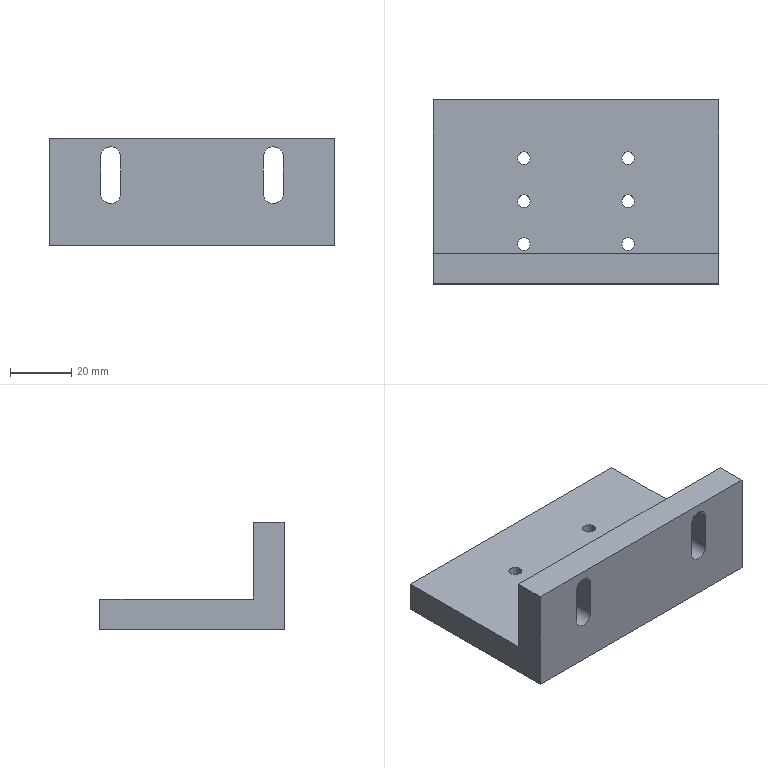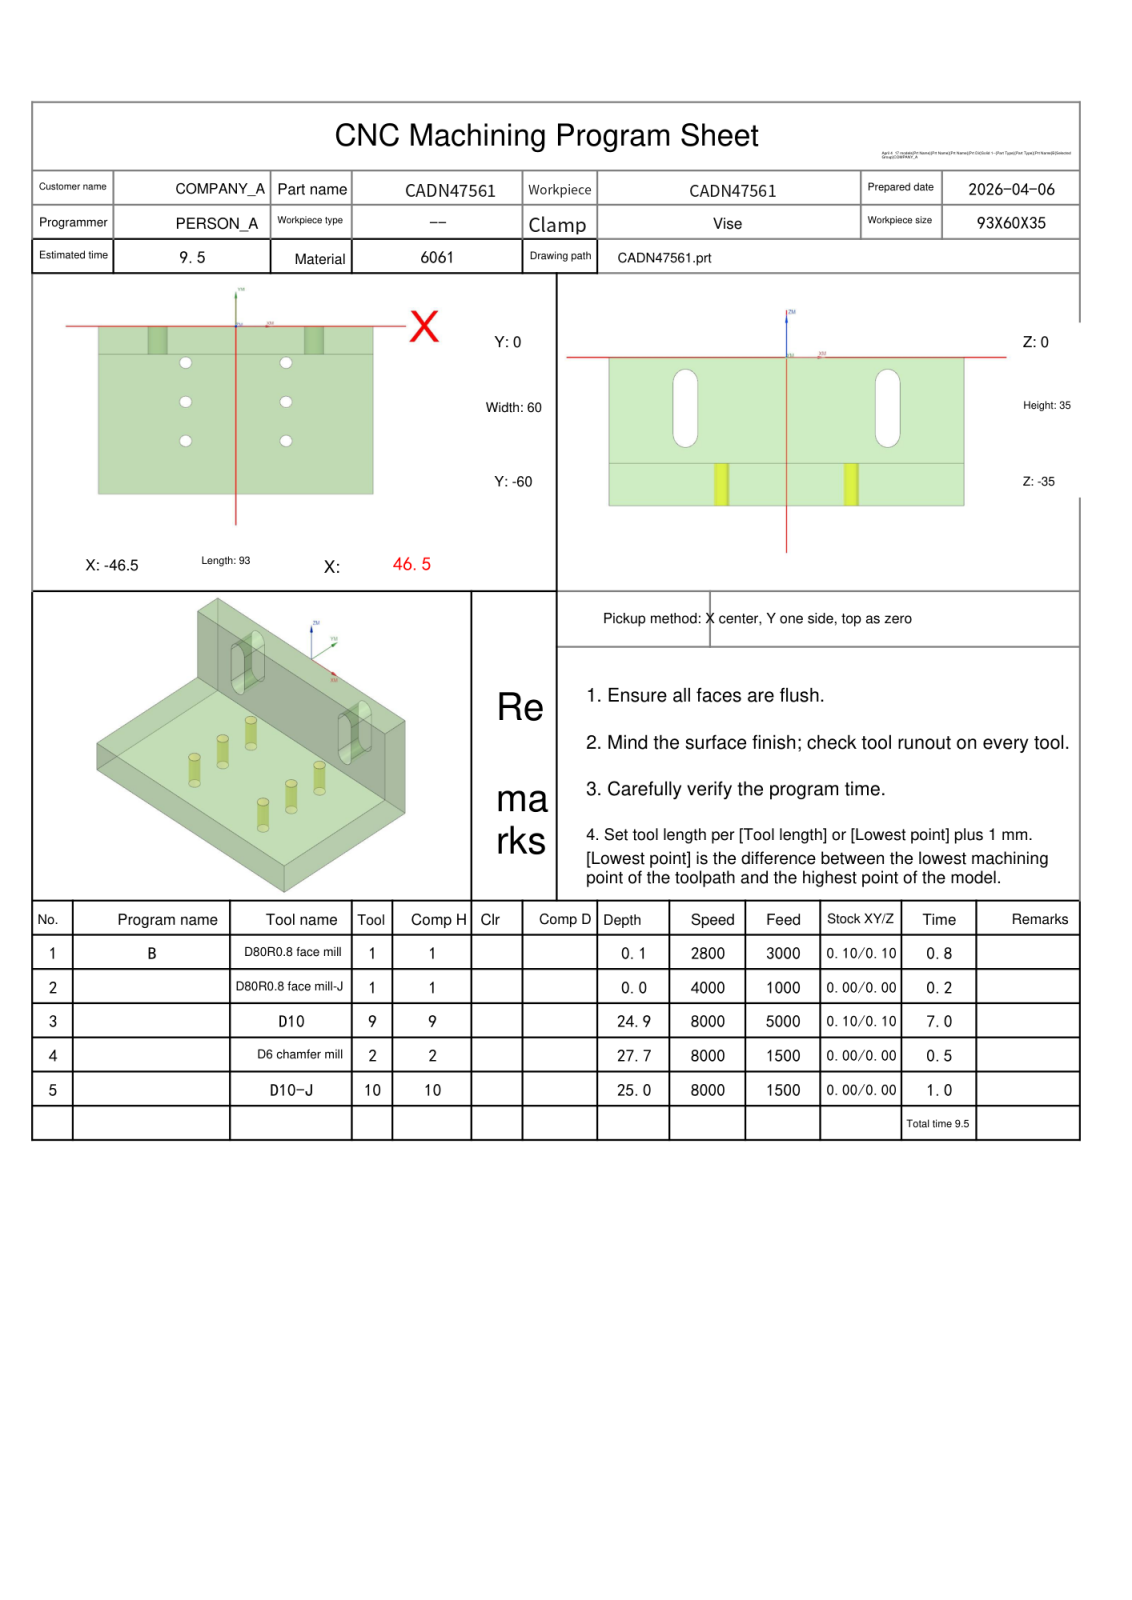NC program | NX | posted by the shop | part box 93 x 60 x 35 mm
Whole program:
%
O0001
(Machine time: 10.28 MIN)
(===Total Tool:4===)
(T1=D80R0.8 face mill D=80.  R=0.8  D-  H01 Z=0.    )
(T9=D10     D=10.  R=0.   D-  H09 Z=-24.9 )
(T2=D6 chamfer mill   D=6.   R=0.   D-  H02 Z=-27.67)
(T10=D10-J  D=10.  R=0.   D10 H10 Z=-25.  )
G80 G90 G17 G49 G40
G91 G28 Z0
M01
N1 T01 M06
(D80R0.8 face mill  D=80. R=0.8 H=01 ce=0.10 di=0.10)
G00 G90 G54 X98.597 Y-30. M03 S2800
G43 H01 Z20.
M08
Z6.011
G01 Z4.011 F3000.
X86.597
X-86.597
X-98.597
Z6.011
G00 X98.597
Z5.522
G01 Z3.522
X86.597
X-86.597
X-98.597
Z5.522
G00 X98.597
Z5.033
G01 Z3.033
X86.597
X-86.597
X-98.597
Z5.033
G00 X98.597
Z4.544
G01 Z2.544
X86.597
X-86.597
X-98.597
Z4.544
G00 Z20.
X98.597
Z4.056
G01 Z2.056
X86.597
X-86.597
X-98.597
Z4.056
G00 Z20.
X98.597
Z3.567
G01 Z1.567
X86.597
X-86.597
X-98.597
Z3.567
G00 Z20.
X98.597
Z3.078
G01 Z1.078
X86.597
X-86.597
X-98.597
Z3.078
G00 Z20.
X98.597
Z2.589
G01 Z.589
X86.597
X-86.597
X-98.597
Z2.589
G00 Z20.
X98.597
Z2.1
G01 Z.1
X86.597
X-86.597
X-98.597
Z2.1
G00 Z20.
G91 G28 Z0.0
M05
M09
G91 G28 Z0.0
M01
N2 T01 M06
(D80R0.8 face mill-J  D=80. R=0.8 H=01 ce=0.00 di=0.00)
G00 G90 G54 X98.499 Y-30. M03 S4000
G43 H01 Z20.
M08
Z2.
G01 Z0.0 F1000.
X86.499
X-86.499
X-98.499
Z2.
G00 Z20.
G91 G28 Z0.0
M05
M09
G91 G28 Z0.0
M01
N3 T09 M06
(D10  D=10. R=0. H=09 ce=0.10 di=0.10)
G00 G90 G54 X54.5 Y-60.1 M03 S8000
G43 H09 Z14.5
M08
Z.907
G01 Z-.593 F5000.
X51.4
X-50.401
G02 X-51.4 Y-59.101 I.001 J1.
G01 Y-53.599
G02 X-50.401 Y-52.6 I1. J-.001
G01 X50.401
G03 X51.4 Y-51.601 I-.001 J1.
G01 Y-46.099
G03 X50.401 Y-45.1 I-1. J-.001
G01 X-50.401
G02 X-51.4 Y-44.101 I.001 J1.
G01 Y-38.599
G02 X-50.401 Y-37.6 I1. J-.001
G01 X50.401
G03 X51.4 Y-36.601 I-.001 J1.
G01 Y-31.099
G03 X50.401 Y-30.1 I-1. J-.001
G01 X-50.401
G02 X-51.4 Y-29.101 I.001 J1.
G01 Y-23.599
G02 X-50.401 Y-22.6 I1. J-.001
G01 X50.544
G03 X51.532 Y-21.755 I-.001 J1.
G01 X52.388 Y-16.254
X52.4 Y-16.1
G03 X51.4 Y-15.1 I-1. J0.0
G01 X-51.4
X-54.6
Z.907
G00 X54.5 Y-60.1
Z.314
G01 Z-1.186
X51.4
X-50.401
G02 X-51.4 Y-59.101 I.001 J1.
G01 Y-53.599
G02 X-50.401 Y-52.6 I1. J-.001
G01 X50.401
G03 X51.4 Y-51.601 I-.001 J1.
G01 Y-46.099
G03 X50.401 Y-45.1 I-1. J-.001
G01 X-50.401
G02 X-51.4 Y-44.101 I.001 J1.
G01 Y-38.599
G02 X-50.401 Y-37.6 I1. J-.001
G01 X50.401
G03 X51.4 Y-36.601 I-.001 J1.
G01 Y-31.099
G03 X50.401 Y-30.1 I-1. J-.001
G01 X-50.401
G02 X-51.4 Y-29.101 I.001 J1.
G01 Y-23.599
G02 X-50.401 Y-22.6 I1. J-.001
G01 X50.544
G03 X51.532 Y-21.755 I-.001 J1.
G01 X52.388 Y-16.254
X52.4 Y-16.1
G03 X51.4 Y-15.1 I-1. J0.0
G01 X-51.4
X-54.6
Z.314
G00 X54.5 Y-60.1
Z-.279
G01 Z-1.779
X51.4
X-50.401
G02 X-51.4 Y-59.101 I.001 J1.
G01 Y-53.599
G02 X-50.401 Y-52.6 I1. J-.001
G01 X50.401
G03 X51.4 Y-51.601 I-.001 J1.
G01 Y-46.099
G03 X50.401 Y-45.1 I-1. J-.001
G01 X-50.401
G02 X-51.4 Y-44.101 I.001 J1.
G01 Y-38.599
G02 X-50.401 Y-37.6 I1. J-.001
G01 X50.401
G03 X51.4 Y-36.601 I-.001 J1.
G01 Y-31.099
G03 X50.401 Y-30.1 I-1. J-.001
G01 X-50.401
G02 X-51.4 Y-29.101 I.001 J1.
G01 Y-23.599
G02 X-50.401 Y-22.6 I1. J-.001
G01 X50.544
G03 X51.532 Y-21.755 I-.001 J1.
G01 X52.388 Y-16.254
X52.4 Y-16.1
G03 X51.4 Y-15.1 I-1. J0.0
G01 X-51.4
X-54.6
Z-.279
G00 X54.5 Y-60.1
Z-.871
G01 Z-2.371
X51.4
X-50.401
G02 X-51.4 Y-59.101 I.001 J1.
G01 Y-53.599
G02 X-50.401 Y-52.6 I1. J-.001
G01 X50.401
G03 X51.4 Y-51.601 I-.001 J1.
G01 Y-46.099
G03 X50.401 Y-45.1 I-1. J-.001
G01 X-50.401
G02 X-51.4 Y-44.101 I.001 J1.
G01 Y-38.599
G02 X-50.401 Y-37.6 I1. J-.001
G01 X50.401
G03 X51.4 Y-36.601 I-.001 J1.
G01 Y-31.099
G03 X50.401 Y-30.1 I-1. J-.001
G01 X-50.401
G02 X-51.4 Y-29.101 I.001 J1.
G01 Y-23.599
G02 X-50.401 Y-22.6 I1. J-.001
G01 X50.544
G03 X51.532 Y-21.755 I-.001 J1.
G01 X52.388 Y-16.254
X52.4 Y-16.1
G03 X51.4 Y-15.1 I-1. J0.0
G01 X-51.4
X-54.6
Z-.871
G00 X54.5 Y-60.1
Z-1.464
G01 Z-2.964
X51.4
X-50.401
G02 X-51.4 Y-59.101 I.001 J1.
G01 Y-53.599
G02 X-50.401 Y-52.6 I1. J-.001
G01 X50.401
G03 X51.4 Y-51.601 I-.001 J1.
G01 Y-46.099
G03 X50.401 Y-45.1 I-1. J-.001
G01 X-50.401
G02 X-51.4 Y-44.101 I.001 J1.
G01 Y-38.599
G02 X-50.401 Y-37.6 I1. J-.001
G01 X50.401
G03 X51.4 Y-36.601 I-.001 J1.
G01 Y-31.099
G03 X50.401 Y-30.1 I-1. J-.001
G01 X-50.401
G02 X-51.4 Y-29.101 I.001 J1.
G01 Y-23.599
G02 X-50.401 Y-22.6 I1. J-.001
G01 X50.544
G03 X51.532 Y-21.755 I-.001 J1.
G01 X52.388 Y-16.254
X52.4 Y-16.1
G03 X51.4 Y-15.1 I-1. J0.0
G01 X-51.4
X-54.6
Z-1.464
G00 X54.5 Y-60.1
Z-2.057
G01 Z-3.557
X51.4
X-50.401
G02 X-51.4 Y-59.101 I.001 J1.
G01 Y-53.599
G02 X-50.401 Y-52.6 I1. J-.001
G01 X50.401
G03 X51.4 Y-51.601 I-.001 J1.
G01 Y-46.099
G03 X50.401 Y-45.1 I-1. J-.001
G01 X-50.401
G02 X-51.4 Y-44.101 I.001 J1.
G01 Y-38.599
G02 X-50.401 Y-37.6 I1. J-.001
G01 X50.401
G03 X51.4 Y-36.601 I-.001 J1.
G01 Y-31.099
G03 X50.401 Y-30.1 I-1. J-.001
G01 X-50.401
G02 X-51.4 Y-29.101 I.001 J1.
G01 Y-23.599
G02 X-50.401 Y-22.6 I1. J-.001
G01 X50.544
G03 X51.532 Y-21.755 I-.001 J1.
G01 X52.388 Y-16.254
X52.4 Y-16.1
G03 X51.4 Y-15.1 I-1. J0.0
G01 X-51.4
X-54.6
Z-2.057
G00 X54.5 Y-60.1
Z-2.65
G01 Z-4.15
X51.4
X-50.401
G02 X-51.4 Y-59.101 I.001 J1.
G01 Y-53.599
G02 X-50.401 Y-52.6 I1. J-.001
G01 X50.401
G03 X51.4 Y-51.601 I-.001 J1.
G01 Y-46.099
G03 X50.401 Y-45.1 I-1. J-.001
G01 X-50.401
G02 X-51.4 Y-44.101 I.001 J1.
G01 Y-38.599
G02 X-50.401 Y-37.6 I1. J-.001
G01 X50.401
G03 X51.4 Y-36.601 I-.001 J1.
G01 Y-31.099
G03 X50.401 Y-30.1 I-1. J-.001
G01 X-50.401
G02 X-51.4 Y-29.101 I.001 J1.
G01 Y-23.599
G02 X-50.401 Y-22.6 I1. J-.001
G01 X50.544
G03 X51.532 Y-21.755 I-.001 J1.
G01 X52.388 Y-16.254
X52.4 Y-16.1
G03 X51.4 Y-15.1 I-1. J0.0
G01 X-51.4
X-54.6
Z-2.65
G00 X54.5 Y-60.1
Z-3.243
G01 Z-4.743
X51.4
X-50.401
G02 X-51.4 Y-59.101 I.001 J1.
G01 Y-53.599
G02 X-50.401 Y-52.6 I1. J-.001
G01 X50.401
G03 X51.4 Y-51.601 I-.001 J1.
G01 Y-46.099
G03 X50.401 Y-45.1 I-1. J-.001
G01 X-50.401
G02 X-51.4 Y-44.101 I.001 J1.
G01 Y-38.599
G02 X-50.401 Y-37.6 I1. J-.001
G01 X50.401
G03 X51.4 Y-36.601 I-.001 J1.
G01 Y-31.099
G03 X50.401 Y-30.1 I-1. J-.001
G01 X-50.401
G02 X-51.4 Y-29.101 I.001 J1.
G01 Y-23.599
G02 X-50.401 Y-22.6 I1. J-.001
G01 X50.544
G03 X51.532 Y-21.755 I-.001 J1.
G01 X52.388 Y-16.254
X52.4 Y-16.1
G03 X51.4 Y-15.1 I-1. J0.0
G01 X-51.4
X-54.6
Z-3.243
G00 X54.5 Y-60.1
Z-3.836
G01 Z-5.336
X51.4
X-50.401
G02 X-51.4 Y-59.101 I.001 J1.
G01 Y-53.599
G02 X-50.401 Y-52.6 I1. J-.001
G01 X50.401
G03 X51.4 Y-51.601 I-.001 J1.
G01 Y-46.099
G03 X50.401 Y-45.1 I-1. J-.001
G01 X-50.401
G02 X-51.4 Y-44.101 I.001 J1.
G01 Y-38.599
G02 X-50.401 Y-37.6 I1. J-.001
G01 X50.401
G03 X51.4 Y-36.601 I-.001 J1.
G01 Y-31.099
G03 X50.401 Y-30.1 I-1. J-.001
G01 X-50.401
G02 X-51.4 Y-29.101 I.001 J1.
G01 Y-23.599
G02 X-50.401 Y-22.6 I1. J-.001
G01 X50.544
G03 X51.532 Y-21.755 I-.001 J1.
G01 X52.388 Y-16.254
X52.4 Y-16.1
G03 X51.4 Y-15.1 I-1. J0.0
G01 X-51.4
X-54.6
Z-3.836
G00 X54.5 Y-60.1
Z-4.429
G01 Z-5.929
X51.4
X-50.401
G02 X-51.4 Y-59.101 I.001 J1.
G01 Y-53.599
G02 X-50.401 Y-52.6 I1. J-.001
G01 X50.401
G03 X51.4 Y-51.601 I-.001 J1.
G01 Y-46.099
G03 X50.401 Y-45.1 I-1. J-.001
G01 X-50.401
G02 X-51.4 Y-44.101 I.001 J1.
G01 Y-38.599
G02 X-50.401 Y-37.6 I1. J-.001
G01 X50.401
G03 X51.4 Y-36.601 I-.001 J1.
G01 Y-31.099
G03 X50.401 Y-30.1 I-1. J-.001
G01 X-50.401
G02 X-51.4 Y-29.101 I.001 J1.
G01 Y-23.599
G02 X-50.401 Y-22.6 I1. J-.001
G01 X50.544
G03 X51.532 Y-21.755 I-.001 J1.
G01 X52.388 Y-16.254
X52.4 Y-16.1
G03 X51.4 Y-15.1 I-1. J0.0
G01 X-51.4
X-54.6
Z-4.429
G00 X54.5 Y-60.1
Z-5.021
G01 Z-6.521
X51.4
X-50.401
G02 X-51.4 Y-59.101 I.001 J1.
G01 Y-53.599
G02 X-50.401 Y-52.6 I1. J-.001
G01 X50.401
G03 X51.4 Y-51.601 I-.001 J1.
G01 Y-46.099
G03 X50.401 Y-45.1 I-1. J-.001
G01 X-50.401
G02 X-51.4 Y-44.101 I.001 J1.
G01 Y-38.599
G02 X-50.401 Y-37.6 I1. J-.001
G01 X50.401
G03 X51.4 Y-36.601 I-.001 J1.
G01 Y-31.099
G03 X50.401 Y-30.1 I-1. J-.001
G01 X-50.401
G02 X-51.4 Y-29.101 I.001 J1.
G01 Y-23.599
G02 X-50.401 Y-22.6 I1. J-.001
G01 X50.544
G03 X51.532 Y-21.755 I-.001 J1.
G01 X52.388 Y-16.254
X52.4 Y-16.1
G03 X51.4 Y-15.1 I-1. J0.0
G01 X-51.4
X-54.6
Z-5.021
G00 X54.5 Y-60.1
Z-5.614
G01 Z-7.114
X51.4
X-50.401
G02 X-51.4 Y-59.101 I.001 J1.
G01 Y-53.599
G02 X-50.401 Y-52.6 I1. J-.001
G01 X50.401
G03 X51.4 Y-51.601 I-.001 J1.
G01 Y-46.099
G03 X50.401 Y-45.1 I-1. J-.001
G01 X-50.401
G02 X-51.4 Y-44.101 I.001 J1.
G01 Y-38.599
G02 X-50.401 Y-37.6 I1. J-.001
G01 X50.401
G03 X51.4 Y-36.601 I-.001 J1.
G01 Y-31.099
G03 X50.401 Y-30.1 I-1. J-.001
G01 X-50.401
G02 X-51.4 Y-29.101 I.001 J1.
G01 Y-23.599
G02 X-50.401 Y-22.6 I1. J-.001
G01 X50.544
G03 X51.532 Y-21.755 I-.001 J1.
G01 X52.388 Y-16.254
X52.4 Y-16.1
G03 X51.4 Y-15.1 I-1. J0.0
G01 X-51.4
X-54.6
Z-5.614
G00 X54.5 Y-60.1
Z-6.207
G01 Z-7.707
X51.4
X-50.401
G02 X-51.4 Y-59.101 I.001 J1.
G01 Y-53.599
G02 X-50.401 Y-52.6 I1. J-.001
G01 X50.401
G03 X51.4 Y-51.601 I-.001 J1.
G01 Y-46.099
G03 X50.401 Y-45.1 I-1. J-.001
G01 X-50.401
G02 X-51.4 Y-44.101 I.001 J1.
G01 Y-38.599
G02 X-50.401 Y-37.6 I1. J-.001
G01 X50.401
G03 X51.4 Y-36.601 I-.001 J1.
G01 Y-31.099
G03 X50.401 Y-30.1 I-1. J-.001
G01 X-50.401
G02 X-51.4 Y-29.101 I.001 J1.
G01 Y-23.599
G02 X-50.401 Y-22.6 I1. J-.001
G01 X50.544
G03 X51.532 Y-21.755 I-.001 J1.
G01 X52.388 Y-16.254
X52.4 Y-16.1
G03 X51.4 Y-15.1 I-1. J0.0
G01 X-51.4
X-54.6
Z-6.207
G00 X54.5 Y-60.1
Z-6.8
G01 Z-8.3
X51.4
X-50.401
G02 X-51.4 Y-59.101 I.001 J1.
G01 Y-53.599
G02 X-50.401 Y-52.6 I1. J-.001
G01 X50.401
G03 X51.4 Y-51.601 I-.001 J1.
G01 Y-46.099
G03 X50.401 Y-45.1 I-1. J-.001
G01 X-50.401
G02 X-51.4 Y-44.101 I.001 J1.
G01 Y-38.599
G02 X-50.401 Y-37.6 I1. J-.001
G01 X50.401
G03 X51.4 Y-36.601 I-.001 J1.
G01 Y-31.099
G03 X50.401 Y-30.1 I-1. J-.001
G01 X-50.401
G02 X-51.4 Y-29.101 I.001 J1.
G01 Y-23.599
G02 X-50.401 Y-22.6 I1. J-.001
G01 X50.544
G03 X51.532 Y-21.755 I-.001 J1.
G01 X52.388 Y-16.254
X52.4 Y-16.1
G03 X51.4 Y-15.1 I-1. J0.0
G01 X-51.4
X-54.6
Z-6.8
G00 X54.5 Y-60.1
Z-7.393
G01 Z-8.893
X51.4
X-50.401
G02 X-51.4 Y-59.101 I.001 J1.
G01 Y-53.599
G02 X-50.401 Y-52.6 I1. J-.001
G01 X50.401
G03 X51.4 Y-51.601 I-.001 J1.
G01 Y-46.099
G03 X50.401 Y-45.1 I-1. J-.001
G01 X-50.401
G02 X-51.4 Y-44.101 I.001 J1.
G01 Y-38.599
G02 X-50.401 Y-37.6 I1. J-.001
G01 X50.401
G03 X51.4 Y-36.601 I-.001 J1.
G01 Y-31.099
G03 X50.401 Y-30.1 I-1. J-.001
G01 X-50.401
G02 X-51.4 Y-29.101 I.001 J1.
G01 Y-23.599
G02 X-50.401 Y-22.6 I1. J-.001
G01 X50.544
G03 X51.532 Y-21.755 I-.001 J1.
G01 X52.388 Y-16.254
X52.4 Y-16.1
G03 X51.4 Y-15.1 I-1. J0.0
G01 X-51.4
X-54.6
Z-7.393
G00 X54.5 Y-60.1
Z-7.986
G01 Z-9.486
X51.4
X-50.401
G02 X-51.4 Y-59.101 I.001 J1.
G01 Y-53.599
G02 X-50.401 Y-52.6 I1. J-.001
G01 X50.401
G03 X51.4 Y-51.601 I-.001 J1.
G01 Y-46.099
G03 X50.401 Y-45.1 I-1. J-.001
G01 X-50.401
G02 X-51.4 Y-44.101 I.001 J1.
G01 Y-38.599
G02 X-50.401 Y-37.6 I1. J-.001
G01 X50.401
G03 X51.4 Y-36.601 I-.001 J1.
G01 Y-31.099
G03 X50.401 Y-30.1 I-1. J-.001
G01 X-50.401
G02 X-51.4 Y-29.101 I.001 J1.
G01 Y-23.599
G02 X-50.401 Y-22.6 I1. J-.001
G01 X50.544
G03 X51.532 Y-21.755 I-.001 J1.
G01 X52.388 Y-16.254
X52.4 Y-16.1
G03 X51.4 Y-15.1 I-1. J0.0
G01 X-51.4
X-54.6
Z-7.986
G00 X54.5 Y-60.1
Z-8.579
G01 Z-10.079
X51.4
X-50.401
G02 X-51.4 Y-59.101 I.001 J1.
G01 Y-53.599
G02 X-50.401 Y-52.6 I1. J-.001
G01 X50.401
G03 X51.4 Y-51.601 I-.001 J1.
G01 Y-46.099
G03 X50.401 Y-45.1 I-1. J-.001
G01 X-50.401
G02 X-51.4 Y-44.101 I.001 J1.
G01 Y-38.599
G02 X-50.401 Y-37.6 I1. J-.001
G01 X50.401
G03 X51.4 Y-36.601 I-.001 J1.
G01 Y-31.099
G03 X50.401 Y-30.1 I-1. J-.001
G01 X-50.401
G02 X-51.4 Y-29.101 I.001 J1.
G01 Y-23.599
G02 X-50.401 Y-22.6 I1. J-.001
G01 X50.544
G03 X51.532 Y-21.755 I-.001 J1.
G01 X52.388 Y-16.254
X52.4 Y-16.1
G03 X51.4 Y-15.1 I-1. J0.0
G01 X-51.4
X-54.6
Z-8.579
G00 X54.5 Y-60.1
Z-9.171
G01 Z-10.671
X51.4
X-50.401
G02 X-51.4 Y-59.101 I.001 J1.
G01 Y-53.599
G02 X-50.401 Y-52.6 I1. J-.001
G01 X50.401
G03 X51.4 Y-51.601 I-.001 J1.
G01 Y-46.099
G03 X50.401 Y-45.1 I-1. J-.001
G01 X-50.401
G02 X-51.4 Y-44.101 I.001 J1.
G01 Y-38.599
G02 X-50.401 Y-37.6 I1. J-.001
G01 X50.401
G03 X51.4 Y-36.601 I-.001 J1.
G01 Y-31.099
G03 X50.401 Y-30.1 I-1. J-.001
G01 X-50.401
G02 X-51.4 Y-29.101 I.001 J1.
G01 Y-23.599
G02 X-50.401 Y-22.6 I1. J-.001
G01 X50.544
G03 X51.532 Y-21.755 I-.001 J1.
G01 X52.388 Y-16.254
X52.4 Y-16.1
G03 X51.4 Y-15.1 I-1. J0.0
G01 X-51.4
X-54.6
Z-9.171
G00 X54.5 Y-60.1
Z-9.764
G01 Z-11.264
X51.4
X-50.401
G02 X-51.4 Y-59.101 I.001 J1.
G01 Y-53.599
G02 X-50.401 Y-52.6 I1. J-.001
G01 X50.401
G03 X51.4 Y-51.601 I-.001 J1.
G01 Y-46.099
G03 X50.401 Y-45.1 I-1. J-.001
G01 X-50.401
G02 X-51.4 Y-44.101 I.001 J1.
G01 Y-38.599
G02 X-50.401 Y-37.6 I1. J-.001
G01 X50.401
G03 X51.4 Y-36.601 I-.001 J1.
G01 Y-31.099
G03 X50.401 Y-30.1 I-1. J-.001
G01 X-50.401
G02 X-51.4 Y-29.101 I.001 J1.
G01 Y-23.599
G02 X-50.401 Y-22.6 I1. J-.001
G01 X50.544
G03 X51.532 Y-21.755 I-.001 J1.
G01 X52.388 Y-16.254
X52.4 Y-16.1
G03 X51.4 Y-15.1 I-1. J0.0
G01 X-51.4
X-54.6
Z-9.764
G00 X54.5 Y-60.1
Z-10.357
G01 Z-11.857
X51.4
X-50.401
G02 X-51.4 Y-59.101 I.001 J1.
G01 Y-53.599
G02 X-50.401 Y-52.6 I1. J-.001
G01 X50.401
G03 X51.4 Y-51.601 I-.001 J1.
G01 Y-46.099
G03 X50.401 Y-45.1 I-1. J-.001
G01 X-50.401
G02 X-51.4 Y-44.101 I.001 J1.
G01 Y-38.599
G02 X-50.401 Y-37.6 I1. J-.001
G01 X50.401
G03 X51.4 Y-36.601 I-.001 J1.
G01 Y-31.099
G03 X50.401 Y-30.1 I-1. J-.001
G01 X-50.401
G02 X-51.4 Y-29.101 I.001 J1.
G01 Y-23.599
G02 X-50.401 Y-22.6 I1. J-.001
G01 X50.544
G03 X51.532 Y-21.755 I-.001 J1.
G01 X52.388 Y-16.254
X52.4 Y-16.1
G03 X51.4 Y-15.1 I-1. J0.0
G01 X-51.4
X-54.6
Z-10.357
G00 X54.5 Y-60.1
Z-10.95
G01 Z-12.45
X51.4
X-50.401
G02 X-51.4 Y-59.101 I.001 J1.
G01 Y-53.599
G02 X-50.401 Y-52.6 I1. J-.001
G01 X50.401
G03 X51.4 Y-51.601 I-.001 J1.
G01 Y-46.099
G03 X50.401 Y-45.1 I-1. J-.001
G01 X-50.401
G02 X-51.4 Y-44.101 I.001 J1.
G01 Y-38.599
G02 X-50.401 Y-37.6 I1. J-.001
G01 X50.401
G03 X51.4 Y-36.601 I-.001 J1.
G01 Y-31.099
G03 X50.401 Y-30.1 I-1. J-.001
G01 X-50.401
G02 X-51.4 Y-29.101 I.001 J1.
G01 Y-23.599
G02 X-50.401 Y-22.6 I1. J-.001
G01 X50.544
G03 X51.532 Y-21.755 I-.001 J1.
G01 X52.388 Y-16.254
X52.4 Y-16.1
G03 X51.4 Y-15.1 I-1. J0.0
G01 X-51.4
X-54.6
Z-10.95
G00 X54.5 Y-60.1
Z-11.543
G01 Z-13.043
X51.4
X-50.401
G02 X-51.4 Y-59.101 I.001 J1.
G01 Y-53.599
G02 X-50.401 Y-52.6 I1. J-.001
G01 X50.401
G03 X51.4 Y-51.601 I-.001 J1.
G01 Y-46.099
G03 X50.401 Y-45.1 I-1. J-.001
G01 X-50.401
G02 X-51.4 Y-44.101 I.001 J1.
G01 Y-38.599
G02 X-50.401 Y-37.6 I1. J-.001
G01 X50.401
G03 X51.4 Y-36.601 I-.001 J1.
G01 Y-31.099
G03 X50.401 Y-30.1 I-1. J-.001
G01 X-50.401
G02 X-51.4 Y-29.101 I.001 J1.
G01 Y-23.599
G02 X-50.401 Y-22.6 I1. J-.001
G01 X50.544
G03 X51.532 Y-21.755 I-.001 J1.
G01 X52.388 Y-16.254
X52.4 Y-16.1
G03 X51.4 Y-15.1 I-1. J0.0
G01 X-51.4
X-54.6
Z-11.543
G00 X54.5 Y-60.1
Z-12.136
G01 Z-13.636
X51.4
X-50.401
G02 X-51.4 Y-59.101 I.001 J1.
G01 Y-53.599
G02 X-50.401 Y-52.6 I1. J-.001
G01 X50.401
G03 X51.4 Y-51.601 I-.001 J1.
G01 Y-46.099
G03 X50.401 Y-45.1 I-1. J-.001
G01 X-50.401
G02 X-51.4 Y-44.101 I.001 J1.
G01 Y-38.599
G02 X-50.401 Y-37.6 I1. J-.001
G01 X50.401
G03 X51.4 Y-36.601 I-.001 J1.
G01 Y-31.099
G03 X50.401 Y-30.1 I-1. J-.001
G01 X-50.401
G02 X-51.4 Y-29.101 I.001 J1.
G01 Y-23.599
G02 X-50.401 Y-22.6 I1. J-.001
G01 X50.544
G03 X51.532 Y-21.755 I-.001 J1.
G01 X52.388 Y-16.254
X52.4 Y-16.1
G03 X51.4 Y-15.1 I-1. J0.0
G01 X-51.4
X-54.6
Z-12.136
G00 X54.5 Y-60.1
Z-12.729
G01 Z-14.229
X51.4
X-50.401
G02 X-51.4 Y-59.101 I.001 J1.
G01 Y-53.599
G02 X-50.401 Y-52.6 I1. J-.001
G01 X50.401
G03 X51.4 Y-51.601 I-.001 J1.
G01 Y-46.099
G03 X50.401 Y-45.1 I-1. J-.001
G01 X-50.401
G02 X-51.4 Y-44.101 I.001 J1.
G01 Y-38.599
G02 X-50.401 Y-37.6 I1. J-.001
G01 X50.401
G03 X51.4 Y-36.601 I-.001 J1.
G01 Y-31.099
G03 X50.401 Y-30.1 I-1. J-.001
G01 X-50.401
G02 X-51.4 Y-29.101 I.001 J1.
G01 Y-23.599
G02 X-50.401 Y-22.6 I1. J-.001
G01 X50.544
G03 X51.532 Y-21.755 I-.001 J1.
G01 X52.388 Y-16.254
X52.4 Y-16.1
G03 X51.4 Y-15.1 I-1. J0.0
G01 X-51.4
X-54.6
Z-12.729
G00 X54.5 Y-60.1
Z-13.321
G01 Z-14.821
X51.4
X-50.401
G02 X-51.4 Y-59.101 I.001 J1.
G01 Y-53.599
G02 X-50.401 Y-52.6 I1. J-.001
G01 X50.401
G03 X51.4 Y-51.601 I-.001 J1.
G01 Y-46.099
G03 X50.401 Y-45.1 I-1. J-.001
G01 X-50.401
G02 X-51.4 Y-44.101 I.001 J1.
G01 Y-38.599
G02 X-50.401 Y-37.6 I1. J-.001
G01 X50.401
G03 X51.4 Y-36.601 I-.001 J1.
G01 Y-31.099
G03 X50.401 Y-30.1 I-1. J-.001
G01 X-50.401
G02 X-51.4 Y-29.101 I.001 J1.
G01 Y-23.599
G02 X-50.401 Y-22.6 I1. J-.001
G01 X50.544
G03 X51.532 Y-21.755 I-.001 J1.
G01 X52.388 Y-16.254
X52.4 Y-16.1
G03 X51.4 Y-15.1 I-1. J0.0
G01 X-51.4
X-54.6
Z-13.321
G00 X54.5 Y-60.1
Z-13.914
G01 Z-15.414
X51.4
X-50.401
G02 X-51.4 Y-59.101 I.001 J1.
G01 Y-53.599
G02 X-50.401 Y-52.6 I1. J-.001
G01 X50.401
G03 X51.4 Y-51.601 I-.001 J1.
G01 Y-46.099
G03 X50.401 Y-45.1 I-1. J-.001
G01 X-50.401
G02 X-51.4 Y-44.101 I.001 J1.
G01 Y-38.599
G02 X-50.401 Y-37.6 I1. J-.001
G01 X50.401
G03 X51.4 Y-36.601 I-.001 J1.
G01 Y-31.099
G03 X50.401 Y-30.1 I-1. J-.001
G01 X-50.401
G02 X-51.4 Y-29.101 I.001 J1.
G01 Y-23.599
G02 X-50.401 Y-22.6 I1. J-.001
G01 X50.544
G03 X51.532 Y-21.755 I-.001 J1.
G01 X52.388 Y-16.254
X52.4 Y-16.1
G03 X51.4 Y-15.1 I-1. J0.0
G01 X-51.4
X-54.6
Z-13.914
G00 X54.5 Y-60.1
Z-14.507
G01 Z-16.007
X51.4
X-50.401
G02 X-51.4 Y-59.101 I.001 J1.
G01 Y-53.599
G02 X-50.401 Y-52.6 I1. J-.001
G01 X50.401
G03 X51.4 Y-51.601 I-.001 J1.
G01 Y-46.099
G03 X50.401 Y-45.1 I-1. J-.001
G01 X-50.401
G02 X-51.4 Y-44.101 I.001 J1.
G01 Y-38.599
G02 X-50.401 Y-37.6 I1. J-.001
G01 X50.401
G03 X51.4 Y-36.601 I-.001 J1.
G01 Y-31.099
G03 X50.401 Y-30.1 I-1. J-.001
G01 X-50.401
G02 X-51.4 Y-29.101 I.001 J1.
G01 Y-23.599
G02 X-50.401 Y-22.6 I1. J-.001
G01 X50.544
G03 X51.532 Y-21.755 I-.001 J1.
G01 X52.388 Y-16.254
X52.4 Y-16.1
G03 X51.4 Y-15.1 I-1. J0.0
G01 X-51.4
X-54.6
Z-14.507
G00 X54.5 Y-60.1
Z-15.1
G01 Z-16.6
X51.4
X-50.401
G02 X-51.4 Y-59.101 I.001 J1.
G01 Y-53.599
G02 X-50.401 Y-52.6 I1. J-.001
G01 X50.401
G03 X51.4 Y-51.601 I-.001 J1.
G01 Y-46.099
G03 X50.401 Y-45.1 I-1. J-.001
G01 X-50.401
G02 X-51.4 Y-44.101 I.001 J1.
G01 Y-38.599
G02 X-50.401 Y-37.6 I1. J-.001
G01 X50.401
G03 X51.4 Y-36.601 I-.001 J1.
G01 Y-31.099
G03 X50.401 Y-30.1 I-1. J-.001
G01 X-50.401
G02 X-51.4 Y-29.101 I.001 J1.
G01 Y-23.599
G02 X-50.401 Y-22.6 I1. J-.001
G01 X50.544
G03 X51.532 Y-21.755 I-.001 J1.
G01 X52.388 Y-16.254
X52.4 Y-16.1
G03 X51.4 Y-15.1 I-1. J0.0
G01 X-51.4
X-54.6
Z-15.1
G00 X54.5 Y-60.1
Z-15.693
G01 Z-17.193
X51.4
X-50.401
G02 X-51.4 Y-59.101 I.001 J1.
G01 Y-53.599
G02 X-50.401 Y-52.6 I1. J-.001
G01 X50.401
G03 X51.4 Y-51.601 I-.001 J1.
G01 Y-46.099
G03 X50.401 Y-45.1 I-1. J-.001
G01 X-50.401
G02 X-51.4 Y-44.101 I.001 J1.
G01 Y-38.599
G02 X-50.401 Y-37.6 I1. J-.001
G01 X50.401
G03 X51.4 Y-36.601 I-.001 J1.
G01 Y-31.099
G03 X50.401 Y-30.1 I-1. J-.001
G01 X-50.401
G02 X-51.4 Y-29.101 I.001 J1.
G01 Y-23.599
G02 X-50.401 Y-22.6 I1. J-.001
G01 X50.544
G03 X51.532 Y-21.755 I-.001 J1.
G01 X52.388 Y-16.254
X52.4 Y-16.1
G03 X51.4 Y-15.1 I-1. J0.0
G01 X-51.4
X-54.6
Z-15.693
G00 X54.5 Y-60.1
Z-16.286
G01 Z-17.786
X51.4
X-50.401
G02 X-51.4 Y-59.101 I.001 J1.
G01 Y-53.599
G02 X-50.401 Y-52.6 I1. J-.001
G01 X50.401
G03 X51.4 Y-51.601 I-.001 J1.
G01 Y-46.099
G03 X50.401 Y-45.1 I-1. J-.001
G01 X-50.401
G02 X-51.4 Y-44.101 I.001 J1.
G01 Y-38.599
G02 X-50.401 Y-37.6 I1. J-.001
G01 X50.401
G03 X51.4 Y-36.601 I-.001 J1.
G01 Y-31.099
G03 X50.401 Y-30.1 I-1. J-.001
G01 X-50.401
G02 X-51.4 Y-29.101 I.001 J1.
G01 Y-23.599
G02 X-50.401 Y-22.6 I1. J-.001
G01 X50.544
G03 X51.532 Y-21.755 I-.001 J1.
G01 X52.388 Y-16.254
X52.4 Y-16.1
G03 X51.4 Y-15.1 I-1. J0.0
G01 X-51.4
X-54.6
Z-16.286
G00 X54.5 Y-60.1
Z-16.879
G01 Z-18.379
X51.4
X-50.401
G02 X-51.4 Y-59.101 I.001 J1.
G01 Y-53.599
G02 X-50.401 Y-52.6 I1. J-.001
G01 X50.401
G03 X51.4 Y-51.601 I-.001 J1.
G01 Y-46.099
G03 X50.401 Y-45.1 I-1. J-.001
G01 X-50.401
G02 X-51.4 Y-44.101 I.001 J1.
G01 Y-38.599
G02 X-50.401 Y-37.6 I1. J-.001
G01 X50.401
G03 X51.4 Y-36.601 I-.001 J1.
G01 Y-31.099
G03 X50.401 Y-30.1 I-1. J-.001
G01 X-50.401
G02 X-51.4 Y-29.101 I.001 J1.
G01 Y-23.599
G02 X-50.401 Y-22.6 I1. J-.001
G01 X50.544
G03 X51.532 Y-21.755 I-.001 J1.
G01 X52.388 Y-16.254
X52.4 Y-16.1
G03 X51.4 Y-15.1 I-1. J0.0
G01 X-51.4
X-54.6
Z-16.879
G00 X54.5 Y-60.1
Z-17.471
G01 Z-18.971
X51.4
X-50.401
G02 X-51.4 Y-59.101 I.001 J1.
G01 Y-53.599
G02 X-50.401 Y-52.6 I1. J-.001
G01 X50.401
G03 X51.4 Y-51.601 I-.001 J1.
G01 Y-46.099
G03 X50.401 Y-45.1 I-1. J-.001
G01 X-50.401
G02 X-51.4 Y-44.101 I.001 J1.
G01 Y-38.599
G02 X-50.401 Y-37.6 I1. J-.001
G01 X50.401
G03 X51.4 Y-36.601 I-.001 J1.
G01 Y-31.099
G03 X50.401 Y-30.1 I-1. J-.001
G01 X-50.401
G02 X-51.4 Y-29.101 I.001 J1.
G01 Y-23.599
G02 X-50.401 Y-22.6 I1. J-.001
G01 X50.544
G03 X51.532 Y-21.755 I-.001 J1.
G01 X52.388 Y-16.254
X52.4 Y-16.1
G03 X51.4 Y-15.1 I-1. J0.0
G01 X-51.4
X-54.6
Z-17.471
G00 X54.5 Y-60.1
Z-18.064
G01 Z-19.564
X51.4
X-50.401
G02 X-51.4 Y-59.101 I.001 J1.
G01 Y-53.599
G02 X-50.401 Y-52.6 I1. J-.001
G01 X50.401
G03 X51.4 Y-51.601 I-.001 J1.
G01 Y-46.099
G03 X50.401 Y-45.1 I-1. J-.001
G01 X-50.401
G02 X-51.4 Y-44.101 I.001 J1.
G01 Y-38.599
G02 X-50.401 Y-37.6 I1. J-.001
G01 X50.401
G03 X51.4 Y-36.601 I-.001 J1.
G01 Y-31.099
G03 X50.401 Y-30.1 I-1. J-.001
G01 X-50.401
G02 X-51.4 Y-29.101 I.001 J1.
G01 Y-23.599
G02 X-50.401 Y-22.6 I1. J-.001
G01 X50.544
G03 X51.532 Y-21.755 I-.001 J1.
G01 X52.388 Y-16.254
X52.4 Y-16.1
G03 X51.4 Y-15.1 I-1. J0.0
G01 X-51.4
X-54.6
Z-18.064
G00 X54.5 Y-60.1
Z-18.657
G01 Z-20.157
X51.4
X-50.401
G02 X-51.4 Y-59.101 I.001 J1.
G01 Y-53.599
G02 X-50.401 Y-52.6 I1. J-.001
G01 X50.401
G03 X51.4 Y-51.601 I-.001 J1.
G01 Y-46.099
G03 X50.401 Y-45.1 I-1. J-.001
G01 X-50.401
G02 X-51.4 Y-44.101 I.001 J1.
G01 Y-38.599
G02 X-50.401 Y-37.6 I1. J-.001
G01 X50.401
G03 X51.4 Y-36.601 I-.001 J1.
G01 Y-31.099
G03 X50.401 Y-30.1 I-1. J-.001
G01 X-50.401
G02 X-51.4 Y-29.101 I.001 J1.
G01 Y-23.599
G02 X-50.401 Y-22.6 I1. J-.001
G01 X50.544
G03 X51.532 Y-21.755 I-.001 J1.
G01 X52.388 Y-16.254
X52.4 Y-16.1
G03 X51.4 Y-15.1 I-1. J0.0
G01 X-51.4
X-54.6
Z-18.657
G00 X54.5 Y-60.1
Z-19.25
G01 Z-20.75
X51.4
X-50.401
G02 X-51.4 Y-59.101 I.001 J1.
G01 Y-53.599
G02 X-50.401 Y-52.6 I1. J-.001
G01 X50.401
G03 X51.4 Y-51.601 I-.001 J1.
G01 Y-46.099
G03 X50.401 Y-45.1 I-1. J-.001
G01 X-50.401
G02 X-51.4 Y-44.101 I.001 J1.
G01 Y-38.599
G02 X-50.401 Y-37.6 I1. J-.001
G01 X50.401
G03 X51.4 Y-36.601 I-.001 J1.
G01 Y-31.099
G03 X50.401 Y-30.1 I-1. J-.001
G01 X-50.401
G02 X-51.4 Y-29.101 I.001 J1.
G01 Y-23.599
G02 X-50.401 Y-22.6 I1. J-.001
G01 X50.544
G03 X51.532 Y-21.755 I-.001 J1.
G01 X52.388 Y-16.254
X52.4 Y-16.1
G03 X51.4 Y-15.1 I-1. J0.0
G01 X-51.4
X-54.6
Z-19.25
G00 X54.5 Y-60.1
Z-19.843
G01 Z-21.343
X51.4
X-50.401
G02 X-51.4 Y-59.101 I.001 J1.
G01 Y-53.599
G02 X-50.401 Y-52.6 I1. J-.001
G01 X50.401
G03 X51.4 Y-51.601 I-.001 J1.
G01 Y-46.099
G03 X50.401 Y-45.1 I-1. J-.001
G01 X-50.401
G02 X-51.4 Y-44.101 I.001 J1.
G01 Y-38.599
G02 X-50.401 Y-37.6 I1. J-.001
G01 X50.401
G03 X51.4 Y-36.601 I-.001 J1.
G01 Y-31.099
G03 X50.401 Y-30.1 I-1. J-.001
G01 X-50.401
G02 X-51.4 Y-29.101 I.001 J1.
G01 Y-23.599
G02 X-50.401 Y-22.6 I1. J-.001
G01 X50.544
G03 X51.532 Y-21.755 I-.001 J1.
G01 X52.388 Y-16.254
X52.4 Y-16.1
G03 X51.4 Y-15.1 I-1. J0.0
G01 X-51.4
X-54.6
Z-19.843
G00 X54.5 Y-60.1
Z-20.436
G01 Z-21.936
X51.4
X-50.401
G02 X-51.4 Y-59.101 I.001 J1.
G01 Y-53.599
G02 X-50.401 Y-52.6 I1. J-.001
G01 X50.401
G03 X51.4 Y-51.601 I-.001 J1.
G01 Y-46.099
G03 X50.401 Y-45.1 I-1. J-.001
G01 X-50.401
G02 X-51.4 Y-44.101 I.001 J1.
G01 Y-38.599
G02 X-50.401 Y-37.6 I1. J-.001
G01 X50.401
G03 X51.4 Y-36.601 I-.001 J1.
G01 Y-31.099
G03 X50.401 Y-30.1 I-1. J-.001
G01 X-50.401
G02 X-51.4 Y-29.101 I.001 J1.
G01 Y-23.599
G02 X-50.401 Y-22.6 I1. J-.001
G01 X50.544
G03 X51.532 Y-21.755 I-.001 J1.
G01 X52.388 Y-16.254
X52.4 Y-16.1
G03 X51.4 Y-15.1 I-1. J0.0
G01 X-51.4
X-54.6
Z-20.436
G00 X54.5 Y-60.1
Z-21.029
G01 Z-22.529
X51.4
X-50.401
G02 X-51.4 Y-59.101 I.001 J1.
G01 Y-53.599
G02 X-50.401 Y-52.6 I1. J-.001
G01 X50.401
G03 X51.4 Y-51.601 I-.001 J1.
G01 Y-46.099
G03 X50.401 Y-45.1 I-1. J-.001
G01 X-50.401
G02 X-51.4 Y-44.101 I.001 J1.
G01 Y-38.599
G02 X-50.401 Y-37.6 I1. J-.001
G01 X50.401
G03 X51.4 Y-36.601 I-.001 J1.
G01 Y-31.099
G03 X50.401 Y-30.1 I-1. J-.001
G01 X-50.401
G02 X-51.4 Y-29.101 I.001 J1.
G01 Y-23.599
G02 X-50.401 Y-22.6 I1. J-.001
G01 X50.544
G03 X51.532 Y-21.755 I-.001 J1.
G01 X52.388 Y-16.254
X52.4 Y-16.1
G03 X51.4 Y-15.1 I-1. J0.0
G01 X-51.4
X-54.6
Z-21.029
G00 X54.5 Y-60.1
Z-21.621
G01 Z-23.121
X51.4
X-50.401
G02 X-51.4 Y-59.101 I.001 J1.
G01 Y-53.599
G02 X-50.401 Y-52.6 I1. J-.001
G01 X50.401
G03 X51.4 Y-51.601 I-.001 J1.
G01 Y-46.099
G03 X50.401 Y-45.1 I-1. J-.001
G01 X-50.401
G02 X-51.4 Y-44.101 I.001 J1.
G01 Y-38.599
G02 X-50.401 Y-37.6 I1. J-.001
G01 X50.401
G03 X51.4 Y-36.601 I-.001 J1.
G01 Y-31.099
G03 X50.401 Y-30.1 I-1. J-.001
G01 X-50.401
G02 X-51.4 Y-29.101 I.001 J1.
G01 Y-23.599
G02 X-50.401 Y-22.6 I1. J-.001
G01 X50.544
G03 X51.532 Y-21.755 I-.001 J1.
G01 X52.388 Y-16.254
X52.4 Y-16.1
G03 X51.4 Y-15.1 I-1. J0.0
G01 X-51.4
X-54.6
Z-21.621
G00 X54.5 Y-60.1
Z-22.214
G01 Z-23.714
X51.4
X-50.401
G02 X-51.4 Y-59.101 I.001 J1.
G01 Y-53.599
G02 X-50.401 Y-52.6 I1. J-.001
G01 X50.401
G03 X51.4 Y-51.601 I-.001 J1.
G01 Y-46.099
G03 X50.401 Y-45.1 I-1. J-.001
G01 X-50.401
G02 X-51.4 Y-44.101 I.001 J1.
G01 Y-38.599
G02 X-50.401 Y-37.6 I1. J-.001
G01 X50.401
G03 X51.4 Y-36.601 I-.001 J1.
G01 Y-31.099
G03 X50.401 Y-30.1 I-1. J-.001
G01 X-50.401
G02 X-51.4 Y-29.101 I.001 J1.
G01 Y-23.599
G02 X-50.401 Y-22.6 I1. J-.001
G01 X50.544
G03 X51.532 Y-21.755 I-.001 J1.
G01 X52.388 Y-16.254
X52.4 Y-16.1
G03 X51.4 Y-15.1 I-1. J0.0
G01 X-51.4
X-54.6
Z-22.214
G00 X54.5 Y-60.1
Z-22.807
G01 Z-24.307
X51.4
X-50.401
G02 X-51.4 Y-59.101 I.001 J1.
G01 Y-53.599
G02 X-50.401 Y-52.6 I1. J-.001
G01 X50.401
G03 X51.4 Y-51.601 I-.001 J1.
G01 Y-46.099
G03 X50.401 Y-45.1 I-1. J-.001
G01 X-50.401
G02 X-51.4 Y-44.101 I.001 J1.
G01 Y-38.599
G02 X-50.401 Y-37.6 I1. J-.001
G01 X50.401
G03 X51.4 Y-36.601 I-.001 J1.
G01 Y-31.099
G03 X50.401 Y-30.1 I-1. J-.001
G01 X-50.401
G02 X-51.4 Y-29.101 I.001 J1.
G01 Y-23.599
G02 X-50.401 Y-22.6 I1. J-.001
G01 X50.544
G03 X51.532 Y-21.755 I-.001 J1.
G01 X52.388 Y-16.254
X52.4 Y-16.1
G03 X51.4 Y-15.1 I-1. J0.0
G01 X-51.4
X-54.6
Z-22.807
G00 X54.5 Y-60.1
Z-23.4
G01 Z-24.9
X51.4
X-50.401
G02 X-51.4 Y-59.101 I.001 J1.
G01 Y-53.599
G02 X-50.401 Y-52.6 I1. J-.001
G01 X50.401
G03 X51.4 Y-51.601 I-.001 J1.
G01 Y-46.099
G03 X50.401 Y-45.1 I-1. J-.001
G01 X-50.401
G02 X-51.4 Y-44.101 I.001 J1.
G01 Y-38.599
G02 X-50.401 Y-37.6 I1. J-.001
G01 X50.401
G03 X51.4 Y-36.601 I-.001 J1.
G01 Y-31.099
G03 X50.401 Y-30.1 I-1. J-.001
G01 X-50.401
G02 X-51.4 Y-29.101 I.001 J1.
G01 Y-23.599
G02 X-50.401 Y-22.6 I1. J-.001
G01 X50.544
G03 X51.532 Y-21.755 I-.001 J1.
G01 X52.388 Y-16.254
X52.4 Y-16.1
G03 X51.4 Y-15.1 I-1. J0.0
G01 X-51.4
X-54.6
Z-23.4
G00 Z14.5
G91 G28 Z0.0
M05
M09
G91 G28 Z0.0
M01
N4 T02 M06
(D6 chamfer mill  D=6. R=0. H=02 ce=0.00 di=0.10)
G00 G90 G54 X-17. Y-41. M03 S8000
G43 H02 Z20.
M08
G98 G81 X-17. Y-41. Z-27.667 R-22. F1000.
Y-27.
X17.
Y-41.
G80
G00 Z20.
G00 G90 X.386 Y-11.127 M03 S8000
Z20.
Z.272
G01 Z-1.2 F1350.
G03 X.1 Y-10.927 I-1.286 J-1.532
G01 X.054 Y-10.897
X0.0 Y-10.9
X-46.5 F1500.
G02 X-47.4 Y-10. I0.0 J.9
G01 Y0.0
G02 X-46.5 Y.9 I.9 J0.0
G01 X46.5
G02 X47.4 Y0.0 I0.0 J-.9
G01 Y-10.
G02 X46.5 Y-10.9 I-.9 J0.0
G01 X0.0
X-.054 Y-10.897
X-.1 Y-10.927
G03 X-.386 Y-11.127 I1. J-1.732
G01 Z.272
G00 Z10.
X47.468 Y-13.058
Z-1.809
G01 Z-26.2 F1350.
X47.408 Y-13.144
X47.4 Y-13.174
Y-60. F1500.
G02 X46.5 Y-60.9 I-.9 J0.0
G01 X-46.5
G02 X-47.4 Y-60. I0.0 J.9
G01 Y-13.149
X-47.405 Y-13.129
X-47.445 Y-13.072
Z-1.815
G00 Z10.
X15.885 Y-13.213
Z-1.815
G01 Z-26.2 F1350.
X15.87 Y-13.282
X15.873 Y-13.302
G03 X17. Y-14.167 I1.127 J.302 F1500.
X17.825 Y-13.825 I0.0 J1.167
G01 X18.011 Y-13.584
X18.127 Y-13.302
X18.13 Y-13.282
X18.115 Y-13.213
Z-1.815
G00 Z10.
X16.007 Y-26.588
Z-24.589
G01 Z-26.2 F1350.
G03 X15.847 Y-26.897 I1.687 J-1.075
G01 X15.823 Y-26.946
X15.833 Y-27.
G03 X17. Y-28.167 I1.167 J0.0 F1500.
X18.167 Y-27. I0.0 J1.167
X17. Y-25.833 I-1.167 J0.0
X15.833 Y-27. I0.0 J-1.167
G01 X15.823 Y-27.054
X15.847 Y-27.103
G03 X16.007 Y-27.412 I1.848 J.765
G01 Z-24.589
G00 Z10.
Y-40.588
Z-24.589
G01 Z-26.2 F1350.
G03 X15.847 Y-40.897 I1.687 J-1.075
G01 X15.823 Y-40.946
X15.833 Y-41.
G03 X17. Y-42.167 I1.167 J0.0 F1500.
X18.167 Y-41. I0.0 J1.167
X17. Y-39.833 I-1.167 J0.0
X15.833 Y-41. I0.0 J-1.167
G01 X15.823 Y-41.054
X15.847 Y-41.103
G03 X16.007 Y-41.412 I1.848 J.765
G01 Z-24.589
G00 Z10.
X-17.993 Y-40.588
Z-24.589
G01 Z-26.2 F1350.
G03 X-18.153 Y-40.897 I1.687 J-1.075
G01 X-18.177 Y-40.946
X-18.167 Y-41.
G03 X-17. Y-42.167 I1.167 J0.0 F1500.
X-15.833 Y-41. I0.0 J1.167
X-17. Y-39.833 I-1.167 J0.0
X-18.167 Y-41. I0.0 J-1.167
G01 X-18.177 Y-41.054
X-18.153 Y-41.103
G03 X-17.993 Y-41.412 I1.848 J.765
G01 Z-24.589
G00 Z10.
Y-26.588
Z-24.589
G01 Z-26.2 F1350.
G03 X-18.153 Y-26.897 I1.687 J-1.075
G01 X-18.177 Y-26.946
X-18.167 Y-27.
G03 X-17. Y-28.167 I1.167 J0.0 F1500.
X-15.833 Y-27. I0.0 J1.167
X-17. Y-25.833 I-1.167 J0.0
X-18.167 Y-27. I0.0 J-1.167
G01 X-18.177 Y-27.054
X-18.153 Y-27.103
G03 X-17.993 Y-27.412 I1.848 J.765
G01 Z-24.589
G00 Z10.
X-18.115 Y-13.213
Z-1.815
G01 Z-26.2 F1350.
X-18.13 Y-13.282
X-18.127 Y-13.302
G03 X-17. Y-14.167 I1.127 J.302 F1500.
X-16.175 Y-13.825 I0.0 J1.167
G01 X-15.989 Y-13.584
X-15.873 Y-13.302
X-15.87 Y-13.282
X-15.885 Y-13.213
Z-1.815
G00 Z20.
G91 G28 Z0.0
M05
M09
G91 G28 Z0.0
M01
N5 T10 M06
(D10-J  D=10. R=0. H=10 ce=0.40 di=0.00)
G00 G90 G54 X53.5 Y-62.999 M03 S7000
G43 H10 Z14.5
M08
Z-23.5
G01 Z-25. F1500.
G03 X51.5 Y-61. I-2. J-.001
G01 X-50.501
G02 X-51.5 Y-60.001 I.001 J1.
G01 Y-57.439
G02 X-50.501 Y-56.44 I1. J-.001
G01 X50.6
G03 X51.5 Y-55.54 I0.0 J.9
G01 Y-52.88
G03 X50.5 Y-51.88 I-1. J0.0
G01 X-50.6
G02 X-51.5 Y-50.98 I0.0 J.9
G01 Y-48.32
G02 X-50.5 Y-47.32 I1. J0.0
G01 X50.6
G03 X51.5 Y-46.42 I0.0 J.9
G01 Y-43.76
G03 X50.5 Y-42.76 I-1. J0.0
G01 X-50.6
G02 X-51.5 Y-41.86 I0.0 J.9
G01 Y-39.2
G02 X-50.5 Y-38.2 I1. J0.0
G01 X50.6
G03 X51.5 Y-37.3 I0.0 J.9
G01 Y-34.64
G03 X50.5 Y-33.64 I-1. J0.0
G01 X-50.6
G02 X-51.5 Y-32.74 I0.0 J.9
G01 Y-30.08
G02 X-50.5 Y-29.08 I1. J0.0
G01 X50.6
G03 X51.5 Y-28.18 I0.0 J.9
G01 Y-25.52
G03 X50.5 Y-24.52 I-1. J0.0
G01 X-50.6
G02 X-51.5 Y-23.62 I0.0 J.9
G01 Y-20.96
G02 X-50.5 Y-19.96 I1. J0.0
G01 X50.6
G03 X51.5 Y-19.06 I0.0 J.9
G01 Y-16.4
G03 X50.5 Y-15.4 I-1. J0.0
G01 X-51.5
G03 X-53.5 Y-17.4 I0.0 J-2.
G01 Z-23.5
G00 Z14.5
G00 G90 X53.5 Y-17.199 M03 S8000
Z14.5
Z-11.5
G01 Z-12.5 F1000.
G41 D10
Y-16.999
G03 X51.5 Y-15. I-2. J-.001
G01 X-51.5
G03 X-53.5 Y-16.999 I0.0 J-2.
G01 G40 Y-17.199
Z-11.5
G00 X53.5
Z-24.
G01 Z-25.
G41 D10
Y-16.999
G03 X51.5 Y-15. I-2. J-.001
G01 X-51.5
G03 X-53.5 Y-16.999 I0.0 J-2.
G01 G40 Y-17.199
Z-24.
G00 Z14.5
M05
M09
G91 G28 Z0.0
G91 G28 Y0.0
M30
%